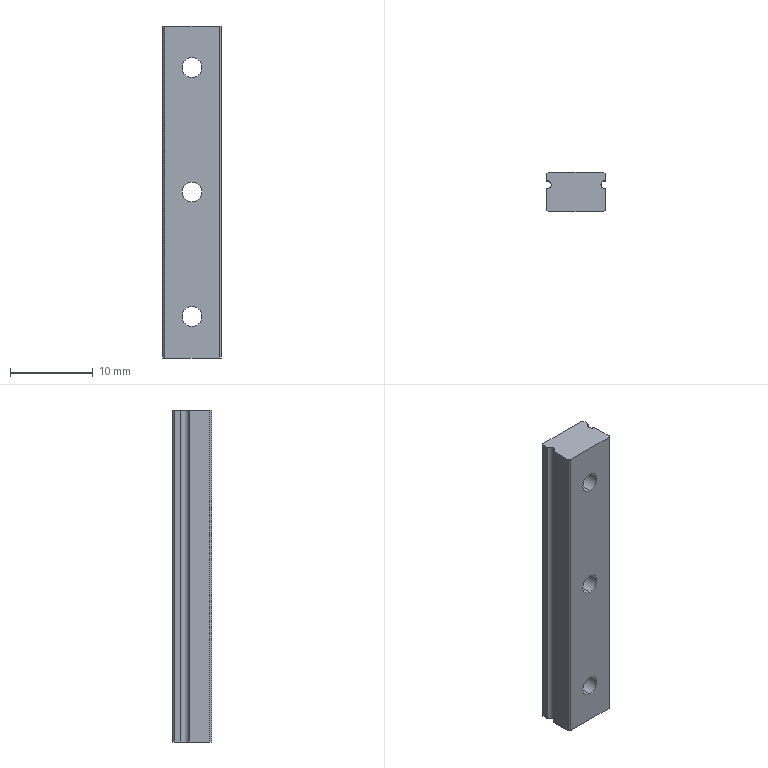Part | SolidWorks | features BaseBody 1 | 1 solid | 30 faces | box 7 x 4.7 x 40 mm | volume 1153 mm3 | cylinder 15 | plane 15 | commonest cylinder face diameters 2.4 x6 4.2 x6 1 x3
STEP:
#1=CARTESIAN_POINT('',(-8.978,1.895,33.8));
#2=VERTEX_POINT('',#1);
#3=CARTESIAN_POINT('',(-8.978,1.895,36.2));
#4=VERTEX_POINT('',#3);
#5=CARTESIAN_POINT('',(-8.978,1.895,35.));
#6=DIRECTION('',(0.,1.,0.));
#7=DIRECTION('',(0.,0.,1.));
#8=AXIS2_PLACEMENT_3D('',#5,#6,#7);
#9=CIRCLE('',#8,1.2);
#10=EDGE_CURVE('',#2,#4,#9,.T.);
#11=ORIENTED_EDGE('',*,*,#10,.F.);
#12=CARTESIAN_POINT('',(-8.978,4.295,33.8));
#13=VERTEX_POINT('',#12);
#14=CARTESIAN_POINT('',(-8.978,-34.284,33.8));
#15=DIRECTION('',(0.,1.,0.));
#16=VECTOR('',#15,1000.);
#17=LINE('',#14,#16);
#18=EDGE_CURVE('',#2,#13,#17,.T.);
#19=ORIENTED_EDGE('',*,*,#18,.T.);
#20=CARTESIAN_POINT('',(-8.978,4.295,36.2));
#21=VERTEX_POINT('',#20);
#22=CARTESIAN_POINT('',(-8.978,4.295,35.));
#23=DIRECTION('',(0.,-1.,0.));
#24=DIRECTION('',(0.,0.,1.));
#25=AXIS2_PLACEMENT_3D('',#22,#23,#24);
#26=CIRCLE('',#25,1.2);
#27=EDGE_CURVE('',#21,#13,#26,.T.);
#28=ORIENTED_EDGE('',*,*,#27,.F.);
#29=CARTESIAN_POINT('',(-8.978,-34.284,36.2));
#30=DIRECTION('',(0.,1.,0.));
#31=VECTOR('',#30,1000.);
#32=LINE('',#29,#31);
#33=EDGE_CURVE('',#4,#21,#32,.T.);
#34=ORIENTED_EDGE('',*,*,#33,.F.);
#35=EDGE_LOOP('',(#11,#19,#28,#34));
#36=FACE_OUTER_BOUND('',#35,.T.);
#37=CARTESIAN_POINT('',(-8.978,-34.284,35.));
#38=DIRECTION('',(0.,1.,0.));
#39=DIRECTION('',(0.,0.,1.));
#40=AXIS2_PLACEMENT_3D('',#37,#38,#39);
#41=CYLINDRICAL_SURFACE('',#40,1.2);
#42=ADVANCED_FACE('',(#36),#41,.F.);
#43=CARTESIAN_POINT('',(-8.978,1.895,18.8));
#44=VERTEX_POINT('',#43);
#45=CARTESIAN_POINT('',(-8.978,1.895,21.2));
#46=VERTEX_POINT('',#45);
#47=CARTESIAN_POINT('',(-8.978,1.895,20.));
#48=DIRECTION('',(0.,1.,0.));
#49=DIRECTION('',(0.,0.,1.));
#50=AXIS2_PLACEMENT_3D('',#47,#48,#49);
#51=CIRCLE('',#50,1.2);
#52=EDGE_CURVE('',#44,#46,#51,.T.);
#53=ORIENTED_EDGE('',*,*,#52,.F.);
#54=CARTESIAN_POINT('',(-8.978,4.295,18.8));
#55=VERTEX_POINT('',#54);
#56=CARTESIAN_POINT('',(-8.978,-34.284,18.8));
#57=DIRECTION('',(0.,1.,0.));
#58=VECTOR('',#57,1000.);
#59=LINE('',#56,#58);
#60=EDGE_CURVE('',#44,#55,#59,.T.);
#61=ORIENTED_EDGE('',*,*,#60,.T.);
#62=CARTESIAN_POINT('',(-8.978,4.295,21.2));
#63=VERTEX_POINT('',#62);
#64=CARTESIAN_POINT('',(-8.978,4.295,20.));
#65=DIRECTION('',(0.,-1.,0.));
#66=DIRECTION('',(0.,0.,1.));
#67=AXIS2_PLACEMENT_3D('',#64,#65,#66);
#68=CIRCLE('',#67,1.2);
#69=EDGE_CURVE('',#63,#55,#68,.T.);
#70=ORIENTED_EDGE('',*,*,#69,.F.);
#71=CARTESIAN_POINT('',(-8.978,-34.284,21.2));
#72=DIRECTION('',(0.,1.,0.));
#73=VECTOR('',#72,1000.);
#74=LINE('',#71,#73);
#75=EDGE_CURVE('',#46,#63,#74,.T.);
#76=ORIENTED_EDGE('',*,*,#75,.F.);
#77=EDGE_LOOP('',(#53,#61,#70,#76));
#78=FACE_OUTER_BOUND('',#77,.T.);
#79=CARTESIAN_POINT('',(-8.978,-34.284,20.));
#80=DIRECTION('',(0.,1.,0.));
#81=DIRECTION('',(0.,0.,1.));
#82=AXIS2_PLACEMENT_3D('',#79,#80,#81);
#83=CYLINDRICAL_SURFACE('',#82,1.2);
#84=ADVANCED_FACE('',(#78),#83,.F.);
#85=CARTESIAN_POINT('',(-8.978,1.895,3.8));
#86=VERTEX_POINT('',#85);
#87=CARTESIAN_POINT('',(-8.978,1.895,6.2));
#88=VERTEX_POINT('',#87);
#89=CARTESIAN_POINT('',(-8.978,1.895,5.));
#90=DIRECTION('',(0.,1.,0.));
#91=DIRECTION('',(0.,0.,1.));
#92=AXIS2_PLACEMENT_3D('',#89,#90,#91);
#93=CIRCLE('',#92,1.2);
#94=EDGE_CURVE('',#86,#88,#93,.T.);
#95=ORIENTED_EDGE('',*,*,#94,.F.);
#96=CARTESIAN_POINT('',(-8.978,4.295,3.8));
#97=VERTEX_POINT('',#96);
#98=CARTESIAN_POINT('',(-8.978,-34.284,3.8));
#99=DIRECTION('',(0.,1.,0.));
#100=VECTOR('',#99,1000.);
#101=LINE('',#98,#100);
#102=EDGE_CURVE('',#86,#97,#101,.T.);
#103=ORIENTED_EDGE('',*,*,#102,.T.);
#104=CARTESIAN_POINT('',(-8.978,4.295,6.2));
#105=VERTEX_POINT('',#104);
#106=CARTESIAN_POINT('',(-8.978,4.295,5.));
#107=DIRECTION('',(0.,-1.,0.));
#108=DIRECTION('',(0.,0.,1.));
#109=AXIS2_PLACEMENT_3D('',#106,#107,#108);
#110=CIRCLE('',#109,1.2);
#111=EDGE_CURVE('',#105,#97,#110,.T.);
#112=ORIENTED_EDGE('',*,*,#111,.F.);
#113=CARTESIAN_POINT('',(-8.978,-34.284,6.2));
#114=DIRECTION('',(0.,1.,0.));
#115=VECTOR('',#114,1000.);
#116=LINE('',#113,#115);
#117=EDGE_CURVE('',#88,#105,#116,.T.);
#118=ORIENTED_EDGE('',*,*,#117,.F.);
#119=EDGE_LOOP('',(#95,#103,#112,#118));
#120=FACE_OUTER_BOUND('',#119,.T.);
#121=CARTESIAN_POINT('',(-8.978,-34.284,5.));
#122=DIRECTION('',(0.,1.,0.));
#123=DIRECTION('',(0.,0.,1.));
#124=AXIS2_PLACEMENT_3D('',#121,#122,#123);
#125=CYLINDRICAL_SURFACE('',#124,1.2);
#126=ADVANCED_FACE('',(#120),#125,.F.);
#127=CARTESIAN_POINT('',(-8.978,4.295,32.9));
#128=VERTEX_POINT('',#127);
#129=CARTESIAN_POINT('',(-8.978,4.295,37.1));
#130=VERTEX_POINT('',#129);
#131=CARTESIAN_POINT('',(-8.978,4.295,35.));
#132=DIRECTION('',(0.,1.,0.));
#133=DIRECTION('',(0.,0.,1.));
#134=AXIS2_PLACEMENT_3D('',#131,#132,#133);
#135=CIRCLE('',#134,2.1);
#136=EDGE_CURVE('',#128,#130,#135,.T.);
#137=ORIENTED_EDGE('',*,*,#136,.F.);
#138=CARTESIAN_POINT('',(-8.978,6.595,32.9));
#139=VERTEX_POINT('',#138);
#140=CARTESIAN_POINT('',(-8.978,5.445,32.9));
#141=DIRECTION('',(0.,1.,0.));
#142=VECTOR('',#141,1000.);
#143=LINE('',#140,#142);
#144=EDGE_CURVE('',#128,#139,#143,.T.);
#145=ORIENTED_EDGE('',*,*,#144,.T.);
#146=CARTESIAN_POINT('',(-8.978,6.595,37.1));
#147=VERTEX_POINT('',#146);
#148=CARTESIAN_POINT('',(-8.978,6.595,35.));
#149=DIRECTION('',(0.,-1.,0.));
#150=DIRECTION('',(0.,0.,1.));
#151=AXIS2_PLACEMENT_3D('',#148,#149,#150);
#152=CIRCLE('',#151,2.1);
#153=EDGE_CURVE('',#147,#139,#152,.T.);
#154=ORIENTED_EDGE('',*,*,#153,.F.);
#155=CARTESIAN_POINT('',(-8.978,5.445,37.1));
#156=DIRECTION('',(0.,1.,0.));
#157=VECTOR('',#156,1000.);
#158=LINE('',#155,#157);
#159=EDGE_CURVE('',#130,#147,#158,.T.);
#160=ORIENTED_EDGE('',*,*,#159,.F.);
#161=EDGE_LOOP('',(#137,#145,#154,#160));
#162=FACE_OUTER_BOUND('',#161,.T.);
#163=CARTESIAN_POINT('',(-8.978,5.445,35.));
#164=DIRECTION('',(0.,1.,0.));
#165=DIRECTION('',(0.,0.,1.));
#166=AXIS2_PLACEMENT_3D('',#163,#164,#165);
#167=CYLINDRICAL_SURFACE('',#166,2.1);
#168=ADVANCED_FACE('',(#162),#167,.F.);
#169=CARTESIAN_POINT('',(-8.978,4.295,17.9));
#170=VERTEX_POINT('',#169);
#171=CARTESIAN_POINT('',(-8.978,4.295,22.1));
#172=VERTEX_POINT('',#171);
#173=CARTESIAN_POINT('',(-8.978,4.295,20.));
#174=DIRECTION('',(0.,1.,0.));
#175=DIRECTION('',(0.,0.,1.));
#176=AXIS2_PLACEMENT_3D('',#173,#174,#175);
#177=CIRCLE('',#176,2.1);
#178=EDGE_CURVE('',#170,#172,#177,.T.);
#179=ORIENTED_EDGE('',*,*,#178,.F.);
#180=CARTESIAN_POINT('',(-8.978,6.595,17.9));
#181=VERTEX_POINT('',#180);
#182=CARTESIAN_POINT('',(-8.978,5.445,17.9));
#183=DIRECTION('',(0.,1.,0.));
#184=VECTOR('',#183,1000.);
#185=LINE('',#182,#184);
#186=EDGE_CURVE('',#170,#181,#185,.T.);
#187=ORIENTED_EDGE('',*,*,#186,.T.);
#188=CARTESIAN_POINT('',(-8.978,6.595,22.1));
#189=VERTEX_POINT('',#188);
#190=CARTESIAN_POINT('',(-8.978,6.595,20.));
#191=DIRECTION('',(0.,-1.,0.));
#192=DIRECTION('',(0.,0.,1.));
#193=AXIS2_PLACEMENT_3D('',#190,#191,#192);
#194=CIRCLE('',#193,2.1);
#195=EDGE_CURVE('',#189,#181,#194,.T.);
#196=ORIENTED_EDGE('',*,*,#195,.F.);
#197=CARTESIAN_POINT('',(-8.978,5.445,22.1));
#198=DIRECTION('',(0.,1.,0.));
#199=VECTOR('',#198,1000.);
#200=LINE('',#197,#199);
#201=EDGE_CURVE('',#172,#189,#200,.T.);
#202=ORIENTED_EDGE('',*,*,#201,.F.);
#203=EDGE_LOOP('',(#179,#187,#196,#202));
#204=FACE_OUTER_BOUND('',#203,.T.);
#205=CARTESIAN_POINT('',(-8.978,5.445,20.));
#206=DIRECTION('',(0.,1.,0.));
#207=DIRECTION('',(0.,0.,1.));
#208=AXIS2_PLACEMENT_3D('',#205,#206,#207);
#209=CYLINDRICAL_SURFACE('',#208,2.1);
#210=ADVANCED_FACE('',(#204),#209,.F.);
#211=CARTESIAN_POINT('',(-8.978,4.295,2.9));
#212=VERTEX_POINT('',#211);
#213=CARTESIAN_POINT('',(-8.978,4.295,7.1));
#214=VERTEX_POINT('',#213);
#215=CARTESIAN_POINT('',(-8.978,4.295,5.));
#216=DIRECTION('',(0.,1.,0.));
#217=DIRECTION('',(0.,0.,1.));
#218=AXIS2_PLACEMENT_3D('',#215,#216,#217);
#219=CIRCLE('',#218,2.1);
#220=EDGE_CURVE('',#212,#214,#219,.T.);
#221=ORIENTED_EDGE('',*,*,#220,.F.);
#222=CARTESIAN_POINT('',(-8.978,6.595,2.9));
#223=VERTEX_POINT('',#222);
#224=CARTESIAN_POINT('',(-8.978,5.445,2.9));
#225=DIRECTION('',(0.,1.,0.));
#226=VECTOR('',#225,1000.);
#227=LINE('',#224,#226);
#228=EDGE_CURVE('',#212,#223,#227,.T.);
#229=ORIENTED_EDGE('',*,*,#228,.T.);
#230=CARTESIAN_POINT('',(-8.978,6.595,7.1));
#231=VERTEX_POINT('',#230);
#232=CARTESIAN_POINT('',(-8.978,6.595,5.));
#233=DIRECTION('',(0.,-1.,0.));
#234=DIRECTION('',(0.,0.,1.));
#235=AXIS2_PLACEMENT_3D('',#232,#233,#234);
#236=CIRCLE('',#235,2.1);
#237=EDGE_CURVE('',#231,#223,#236,.T.);
#238=ORIENTED_EDGE('',*,*,#237,.F.);
#239=CARTESIAN_POINT('',(-8.978,5.445,7.1));
#240=DIRECTION('',(0.,1.,0.));
#241=VECTOR('',#240,1000.);
#242=LINE('',#239,#241);
#243=EDGE_CURVE('',#214,#231,#242,.T.);
#244=ORIENTED_EDGE('',*,*,#243,.F.);
#245=EDGE_LOOP('',(#221,#229,#238,#244));
#246=FACE_OUTER_BOUND('',#245,.T.);
#247=CARTESIAN_POINT('',(-8.978,5.445,5.));
#248=DIRECTION('',(0.,1.,0.));
#249=DIRECTION('',(0.,0.,1.));
#250=AXIS2_PLACEMENT_3D('',#247,#248,#249);
#251=CYLINDRICAL_SURFACE('',#250,2.1);
#252=ADVANCED_FACE('',(#246),#251,.F.);
#253=CARTESIAN_POINT('',(-5.978,5.095,40.));
#254=VERTEX_POINT('',#253);
#255=CARTESIAN_POINT('',(-5.478,5.595,40.));
#256=VERTEX_POINT('',#255);
#257=CARTESIAN_POINT('',(-5.478,5.095,40.));
#258=DIRECTION('',(0.,0.,-1.));
#259=DIRECTION('',(-1.,0.,0.));
#260=AXIS2_PLACEMENT_3D('',#257,#258,#259);
#261=CIRCLE('',#260,0.5);
#262=EDGE_CURVE('',#254,#256,#261,.T.);
#263=ORIENTED_EDGE('',*,*,#262,.F.);
#264=CARTESIAN_POINT('',(-5.978,5.095,0.));
#265=VERTEX_POINT('',#264);
#266=CARTESIAN_POINT('',(-5.978,5.095,40.));
#267=DIRECTION('',(0.,0.,-1.));
#268=VECTOR('',#267,1000.);
#269=LINE('',#266,#268);
#270=EDGE_CURVE('',#254,#265,#269,.T.);
#271=ORIENTED_EDGE('',*,*,#270,.T.);
#272=CARTESIAN_POINT('',(-5.478,5.595,0.));
#273=VERTEX_POINT('',#272);
#274=CARTESIAN_POINT('',(-5.478,5.095,0.));
#275=DIRECTION('',(0.,0.,1.));
#276=DIRECTION('',(-1.,0.,0.));
#277=AXIS2_PLACEMENT_3D('',#274,#275,#276);
#278=CIRCLE('',#277,0.5);
#279=EDGE_CURVE('',#273,#265,#278,.T.);
#280=ORIENTED_EDGE('',*,*,#279,.F.);
#281=CARTESIAN_POINT('',(-5.478,5.595,40.));
#282=DIRECTION('',(0.,0.,-1.));
#283=VECTOR('',#282,1000.);
#284=LINE('',#281,#283);
#285=EDGE_CURVE('',#256,#273,#284,.T.);
#286=ORIENTED_EDGE('',*,*,#285,.F.);
#287=EDGE_LOOP('',(#263,#271,#280,#286));
#288=FACE_OUTER_BOUND('',#287,.T.);
#289=CARTESIAN_POINT('',(-5.478,5.095,40.));
#290=DIRECTION('',(0.,0.,-1.));
#291=DIRECTION('',(-1.,0.,0.));
#292=AXIS2_PLACEMENT_3D('',#289,#290,#291);
#293=CYLINDRICAL_SURFACE('',#292,0.5);
#294=ADVANCED_FACE('',(#288),#293,.F.);
#295=CARTESIAN_POINT('',(-8.978,1.895,35.));
#296=DIRECTION('',(0.,1.,0.));
#297=DIRECTION('',(0.,0.,1.));
#298=AXIS2_PLACEMENT_3D('',#295,#296,#297);
#299=CIRCLE('',#298,1.2);
#300=EDGE_CURVE('',#4,#2,#299,.T.);
#301=ORIENTED_EDGE('',*,*,#300,.T.);
#302=ORIENTED_EDGE('',*,*,#10,.T.);
#303=EDGE_LOOP('',(#301,#302));
#304=FACE_BOUND('',#303,.T.);
#305=CARTESIAN_POINT('',(-8.978,1.895,20.));
#306=DIRECTION('',(0.,1.,0.));
#307=DIRECTION('',(0.,0.,1.));
#308=AXIS2_PLACEMENT_3D('',#305,#306,#307);
#309=CIRCLE('',#308,1.2);
#310=EDGE_CURVE('',#46,#44,#309,.T.);
#311=ORIENTED_EDGE('',*,*,#310,.T.);
#312=ORIENTED_EDGE('',*,*,#52,.T.);
#313=EDGE_LOOP('',(#311,#312));
#314=FACE_BOUND('',#313,.T.);
#315=CARTESIAN_POINT('',(-8.978,1.895,5.));
#316=DIRECTION('',(0.,1.,0.));
#317=DIRECTION('',(0.,0.,1.));
#318=AXIS2_PLACEMENT_3D('',#315,#316,#317);
#319=CIRCLE('',#318,1.2);
#320=EDGE_CURVE('',#88,#86,#319,.T.);
#321=ORIENTED_EDGE('',*,*,#320,.T.);
#322=ORIENTED_EDGE('',*,*,#94,.T.);
#323=EDGE_LOOP('',(#321,#322));
#324=FACE_BOUND('',#323,.T.);
#325=CARTESIAN_POINT('',(-12.278,1.895,40.));
#326=VERTEX_POINT('',#325);
#327=CARTESIAN_POINT('',(-12.278,1.895,0.));
#328=VERTEX_POINT('',#327);
#329=CARTESIAN_POINT('',(-12.278,1.895,0.));
#330=DIRECTION('',(0.,0.,-1.));
#331=VECTOR('',#330,1000.);
#332=LINE('',#329,#331);
#333=EDGE_CURVE('',#326,#328,#332,.T.);
#334=ORIENTED_EDGE('',*,*,#333,.T.);
#335=CARTESIAN_POINT('',(-5.678,1.895,0.));
#336=VERTEX_POINT('',#335);
#337=CARTESIAN_POINT('',(-5.478,1.895,0.));
#338=DIRECTION('',(1.,0.,0.));
#339=VECTOR('',#338,1000.);
#340=LINE('',#337,#339);
#341=EDGE_CURVE('',#328,#336,#340,.T.);
#342=ORIENTED_EDGE('',*,*,#341,.T.);
#343=CARTESIAN_POINT('',(-5.678,1.895,40.));
#344=VERTEX_POINT('',#343);
#345=CARTESIAN_POINT('',(-5.678,1.895,0.));
#346=DIRECTION('',(0.,0.,1.));
#347=VECTOR('',#346,1000.);
#348=LINE('',#345,#347);
#349=EDGE_CURVE('',#336,#344,#348,.T.);
#350=ORIENTED_EDGE('',*,*,#349,.T.);
#351=CARTESIAN_POINT('',(-5.478,1.895,40.));
#352=DIRECTION('',(-1.,0.,0.));
#353=VECTOR('',#352,1000.);
#354=LINE('',#351,#353);
#355=EDGE_CURVE('',#344,#326,#354,.T.);
#356=ORIENTED_EDGE('',*,*,#355,.T.);
#357=EDGE_LOOP('',(#334,#342,#350,#356));
#358=FACE_OUTER_BOUND('',#357,.T.);
#359=CARTESIAN_POINT('',(-5.478,1.895,0.));
#360=DIRECTION('',(0.,-1.,0.));
#361=DIRECTION('',(0.,0.,-1.));
#362=AXIS2_PLACEMENT_3D('',#359,#360,#361);
#363=PLANE('',#362);
#364=ADVANCED_FACE('',(#304,#314,#324,#358),#363,.T.);
#365=ORIENTED_EDGE('',*,*,#18,.F.);
#366=ORIENTED_EDGE('',*,*,#300,.F.);
#367=ORIENTED_EDGE('',*,*,#33,.T.);
#368=CARTESIAN_POINT('',(-8.978,4.295,35.));
#369=DIRECTION('',(0.,-1.,0.));
#370=DIRECTION('',(0.,0.,1.));
#371=AXIS2_PLACEMENT_3D('',#368,#369,#370);
#372=CIRCLE('',#371,1.2);
#373=EDGE_CURVE('',#13,#21,#372,.T.);
#374=ORIENTED_EDGE('',*,*,#373,.F.);
#375=EDGE_LOOP('',(#365,#366,#367,#374));
#376=FACE_OUTER_BOUND('',#375,.T.);
#377=CARTESIAN_POINT('',(-8.978,-34.284,35.));
#378=DIRECTION('',(0.,1.,0.));
#379=DIRECTION('',(0.,0.,1.));
#380=AXIS2_PLACEMENT_3D('',#377,#378,#379);
#381=CYLINDRICAL_SURFACE('',#380,1.2);
#382=ADVANCED_FACE('',(#376),#381,.F.);
#383=ORIENTED_EDGE('',*,*,#60,.F.);
#384=ORIENTED_EDGE('',*,*,#310,.F.);
#385=ORIENTED_EDGE('',*,*,#75,.T.);
#386=CARTESIAN_POINT('',(-8.978,4.295,20.));
#387=DIRECTION('',(0.,-1.,0.));
#388=DIRECTION('',(0.,0.,1.));
#389=AXIS2_PLACEMENT_3D('',#386,#387,#388);
#390=CIRCLE('',#389,1.2);
#391=EDGE_CURVE('',#55,#63,#390,.T.);
#392=ORIENTED_EDGE('',*,*,#391,.F.);
#393=EDGE_LOOP('',(#383,#384,#385,#392));
#394=FACE_OUTER_BOUND('',#393,.T.);
#395=CARTESIAN_POINT('',(-8.978,-34.284,20.));
#396=DIRECTION('',(0.,1.,0.));
#397=DIRECTION('',(0.,0.,1.));
#398=AXIS2_PLACEMENT_3D('',#395,#396,#397);
#399=CYLINDRICAL_SURFACE('',#398,1.2);
#400=ADVANCED_FACE('',(#394),#399,.F.);
#401=ORIENTED_EDGE('',*,*,#102,.F.);
#402=ORIENTED_EDGE('',*,*,#320,.F.);
#403=ORIENTED_EDGE('',*,*,#117,.T.);
#404=CARTESIAN_POINT('',(-8.978,4.295,5.));
#405=DIRECTION('',(0.,-1.,0.));
#406=DIRECTION('',(0.,0.,1.));
#407=AXIS2_PLACEMENT_3D('',#404,#405,#406);
#408=CIRCLE('',#407,1.2);
#409=EDGE_CURVE('',#97,#105,#408,.T.);
#410=ORIENTED_EDGE('',*,*,#409,.F.);
#411=EDGE_LOOP('',(#401,#402,#403,#410));
#412=FACE_OUTER_BOUND('',#411,.T.);
#413=CARTESIAN_POINT('',(-8.978,-34.284,5.));
#414=DIRECTION('',(0.,1.,0.));
#415=DIRECTION('',(0.,0.,1.));
#416=AXIS2_PLACEMENT_3D('',#413,#414,#415);
#417=CYLINDRICAL_SURFACE('',#416,1.2);
#418=ADVANCED_FACE('',(#412),#417,.F.);
#419=ORIENTED_EDGE('',*,*,#341,.F.);
#420=CARTESIAN_POINT('',(-12.478,2.095,0.));
#421=VERTEX_POINT('',#420);
#422=CARTESIAN_POINT('',(-12.478,2.095,0.));
#423=DIRECTION('',(0.7071,-0.7071,0.));
#424=VECTOR('',#423,1000.);
#425=LINE('',#422,#424);
#426=EDGE_CURVE('',#421,#328,#425,.T.);
#427=ORIENTED_EDGE('',*,*,#426,.F.);
#428=CARTESIAN_POINT('',(-12.478,4.595,0.));
#429=VERTEX_POINT('',#428);
#430=CARTESIAN_POINT('',(-12.478,4.245,0.));
#431=DIRECTION('',(0.,-1.,0.));
#432=VECTOR('',#431,1000.);
#433=LINE('',#430,#432);
#434=EDGE_CURVE('',#429,#421,#433,.T.);
#435=ORIENTED_EDGE('',*,*,#434,.F.);
#436=CARTESIAN_POINT('',(-12.478,5.595,0.));
#437=VERTEX_POINT('',#436);
#438=CARTESIAN_POINT('',(-12.478,5.095,0.));
#439=DIRECTION('',(0.,0.,1.));
#440=DIRECTION('',(-1.,0.,0.));
#441=AXIS2_PLACEMENT_3D('',#438,#439,#440);
#442=CIRCLE('',#441,0.5);
#443=EDGE_CURVE('',#429,#437,#442,.T.);
#444=ORIENTED_EDGE('',*,*,#443,.T.);
#445=CARTESIAN_POINT('',(-12.478,6.395,0.));
#446=VERTEX_POINT('',#445);
#447=CARTESIAN_POINT('',(-12.478,1.895,0.));
#448=DIRECTION('',(0.,-1.,0.));
#449=VECTOR('',#448,1000.);
#450=LINE('',#447,#449);
#451=EDGE_CURVE('',#446,#437,#450,.T.);
#452=ORIENTED_EDGE('',*,*,#451,.F.);
#453=CARTESIAN_POINT('',(-12.278,6.595,0.));
#454=VERTEX_POINT('',#453);
#455=CARTESIAN_POINT('',(-12.378,6.495,0.));
#456=DIRECTION('',(-0.7071,-0.7071,0.));
#457=VECTOR('',#456,1000.);
#458=LINE('',#455,#457);
#459=EDGE_CURVE('',#454,#446,#458,.T.);
#460=ORIENTED_EDGE('',*,*,#459,.F.);
#461=CARTESIAN_POINT('',(-5.678,6.595,0.));
#462=VERTEX_POINT('',#461);
#463=CARTESIAN_POINT('',(-8.978,6.595,0.));
#464=DIRECTION('',(-1.,0.,0.));
#465=VECTOR('',#464,1000.);
#466=LINE('',#463,#465);
#467=EDGE_CURVE('',#462,#454,#466,.T.);
#468=ORIENTED_EDGE('',*,*,#467,.F.);
#469=CARTESIAN_POINT('',(-5.478,6.395,0.));
#470=VERTEX_POINT('',#469);
#471=CARTESIAN_POINT('',(-5.578,6.495,0.));
#472=DIRECTION('',(-0.7071,0.7071,0.));
#473=VECTOR('',#472,1000.);
#474=LINE('',#471,#473);
#475=EDGE_CURVE('',#470,#462,#474,.T.);
#476=ORIENTED_EDGE('',*,*,#475,.F.);
#477=CARTESIAN_POINT('',(-5.478,6.595,0.));
#478=DIRECTION('',(0.,1.,0.));
#479=VECTOR('',#478,1000.);
#480=LINE('',#477,#479);
#481=EDGE_CURVE('',#273,#470,#480,.T.);
#482=ORIENTED_EDGE('',*,*,#481,.F.);
#483=ORIENTED_EDGE('',*,*,#279,.T.);
#484=CARTESIAN_POINT('',(-5.478,4.595,0.));
#485=VERTEX_POINT('',#484);
#486=CARTESIAN_POINT('',(-5.478,5.095,0.));
#487=DIRECTION('',(0.,0.,1.));
#488=DIRECTION('',(-1.,0.,0.));
#489=AXIS2_PLACEMENT_3D('',#486,#487,#488);
#490=CIRCLE('',#489,0.5);
#491=EDGE_CURVE('',#265,#485,#490,.T.);
#492=ORIENTED_EDGE('',*,*,#491,.T.);
#493=CARTESIAN_POINT('',(-5.478,2.095,0.));
#494=VERTEX_POINT('',#493);
#495=CARTESIAN_POINT('',(-5.478,4.245,0.));
#496=DIRECTION('',(0.,1.,0.));
#497=VECTOR('',#496,1000.);
#498=LINE('',#495,#497);
#499=EDGE_CURVE('',#494,#485,#498,.T.);
#500=ORIENTED_EDGE('',*,*,#499,.F.);
#501=CARTESIAN_POINT('',(-5.678,1.895,0.));
#502=DIRECTION('',(0.7071,0.7071,0.));
#503=VECTOR('',#502,1000.);
#504=LINE('',#501,#503);
#505=EDGE_CURVE('',#336,#494,#504,.T.);
#506=ORIENTED_EDGE('',*,*,#505,.F.);
#507=EDGE_LOOP('',(#419,#427,#435,#444,#452,#460,#468,#476,#482,#483,#492,#500,#506));
#508=FACE_OUTER_BOUND('',#507,.T.);
#509=CARTESIAN_POINT('',(-8.978,4.245,0.));
#510=DIRECTION('',(0.,0.,1.));
#511=DIRECTION('',(1.,0.,0.));
#512=AXIS2_PLACEMENT_3D('',#509,#510,#511);
#513=PLANE('',#512);
#514=ADVANCED_FACE('',(#508),#513,.F.);
#515=ORIENTED_EDGE('',*,*,#426,.T.);
#516=ORIENTED_EDGE('',*,*,#333,.F.);
#517=CARTESIAN_POINT('',(-12.478,2.095,40.));
#518=VERTEX_POINT('',#517);
#519=CARTESIAN_POINT('',(-12.378,1.995,40.));
#520=DIRECTION('',(-0.7071,0.7071,0.));
#521=VECTOR('',#520,1000.);
#522=LINE('',#519,#521);
#523=EDGE_CURVE('',#326,#518,#522,.T.);
#524=ORIENTED_EDGE('',*,*,#523,.T.);
#525=CARTESIAN_POINT('',(-12.478,2.095,0.));
#526=DIRECTION('',(0.,0.,-1.));
#527=VECTOR('',#526,1000.);
#528=LINE('',#525,#527);
#529=EDGE_CURVE('',#518,#421,#528,.T.);
#530=ORIENTED_EDGE('',*,*,#529,.T.);
#531=EDGE_LOOP('',(#515,#516,#524,#530));
#532=FACE_OUTER_BOUND('',#531,.T.);
#533=CARTESIAN_POINT('',(-12.378,1.995,0.));
#534=DIRECTION('',(-0.7071,-0.7071,0.));
#535=DIRECTION('',(0.7071,-0.7071,0.));
#536=AXIS2_PLACEMENT_3D('',#533,#534,#535);
#537=PLANE('',#536);
#538=ADVANCED_FACE('',(#532),#537,.T.);
#539=ORIENTED_EDGE('',*,*,#523,.F.);
#540=ORIENTED_EDGE('',*,*,#355,.F.);
#541=CARTESIAN_POINT('',(-5.478,2.095,40.));
#542=VERTEX_POINT('',#541);
#543=CARTESIAN_POINT('',(-5.678,1.895,40.));
#544=DIRECTION('',(0.7071,0.7071,0.));
#545=VECTOR('',#544,1000.);
#546=LINE('',#543,#545);
#547=EDGE_CURVE('',#344,#542,#546,.T.);
#548=ORIENTED_EDGE('',*,*,#547,.T.);
#549=CARTESIAN_POINT('',(-5.478,4.595,40.));
#550=VERTEX_POINT('',#549);
#551=CARTESIAN_POINT('',(-5.478,4.245,40.));
#552=DIRECTION('',(0.,1.,0.));
#553=VECTOR('',#552,1000.);
#554=LINE('',#551,#553);
#555=EDGE_CURVE('',#542,#550,#554,.T.);
#556=ORIENTED_EDGE('',*,*,#555,.T.);
#557=CARTESIAN_POINT('',(-5.478,5.095,40.));
#558=DIRECTION('',(0.,0.,-1.));
#559=DIRECTION('',(-1.,0.,0.));
#560=AXIS2_PLACEMENT_3D('',#557,#558,#559);
#561=CIRCLE('',#560,0.5);
#562=EDGE_CURVE('',#550,#254,#561,.T.);
#563=ORIENTED_EDGE('',*,*,#562,.T.);
#564=ORIENTED_EDGE('',*,*,#262,.T.);
#565=CARTESIAN_POINT('',(-5.478,6.395,40.));
#566=VERTEX_POINT('',#565);
#567=CARTESIAN_POINT('',(-5.478,6.595,40.));
#568=DIRECTION('',(0.,-1.,0.));
#569=VECTOR('',#568,1000.);
#570=LINE('',#567,#569);
#571=EDGE_CURVE('',#566,#256,#570,.T.);
#572=ORIENTED_EDGE('',*,*,#571,.F.);
#573=CARTESIAN_POINT('',(-5.678,6.595,40.));
#574=VERTEX_POINT('',#573);
#575=CARTESIAN_POINT('',(-5.578,6.495,40.));
#576=DIRECTION('',(0.7071,-0.7071,0.));
#577=VECTOR('',#576,1000.);
#578=LINE('',#575,#577);
#579=EDGE_CURVE('',#574,#566,#578,.T.);
#580=ORIENTED_EDGE('',*,*,#579,.F.);
#581=CARTESIAN_POINT('',(-12.278,6.595,40.));
#582=VERTEX_POINT('',#581);
#583=CARTESIAN_POINT('',(-8.978,6.595,40.));
#584=DIRECTION('',(-1.,0.,0.));
#585=VECTOR('',#584,1000.);
#586=LINE('',#583,#585);
#587=EDGE_CURVE('',#574,#582,#586,.T.);
#588=ORIENTED_EDGE('',*,*,#587,.T.);
#589=CARTESIAN_POINT('',(-12.478,6.395,40.));
#590=VERTEX_POINT('',#589);
#591=CARTESIAN_POINT('',(-12.378,6.495,40.));
#592=DIRECTION('',(0.7071,0.7071,0.));
#593=VECTOR('',#592,1000.);
#594=LINE('',#591,#593);
#595=EDGE_CURVE('',#590,#582,#594,.T.);
#596=ORIENTED_EDGE('',*,*,#595,.F.);
#597=CARTESIAN_POINT('',(-12.478,5.595,40.));
#598=VERTEX_POINT('',#597);
#599=CARTESIAN_POINT('',(-12.478,1.895,40.));
#600=DIRECTION('',(0.,1.,0.));
#601=VECTOR('',#600,1000.);
#602=LINE('',#599,#601);
#603=EDGE_CURVE('',#598,#590,#602,.T.);
#604=ORIENTED_EDGE('',*,*,#603,.F.);
#605=CARTESIAN_POINT('',(-12.478,4.595,40.));
#606=VERTEX_POINT('',#605);
#607=CARTESIAN_POINT('',(-12.478,5.095,40.));
#608=DIRECTION('',(0.,0.,-1.));
#609=DIRECTION('',(-1.,0.,0.));
#610=AXIS2_PLACEMENT_3D('',#607,#608,#609);
#611=CIRCLE('',#610,0.5);
#612=EDGE_CURVE('',#598,#606,#611,.T.);
#613=ORIENTED_EDGE('',*,*,#612,.T.);
#614=CARTESIAN_POINT('',(-12.478,4.245,40.));
#615=DIRECTION('',(0.,-1.,0.));
#616=VECTOR('',#615,1000.);
#617=LINE('',#614,#616);
#618=EDGE_CURVE('',#606,#518,#617,.T.);
#619=ORIENTED_EDGE('',*,*,#618,.T.);
#620=EDGE_LOOP('',(#539,#540,#548,#556,#563,#564,#572,#580,#588,#596,#604,#613,#619));
#621=FACE_OUTER_BOUND('',#620,.T.);
#622=CARTESIAN_POINT('',(-8.978,4.245,40.));
#623=DIRECTION('',(0.,0.,1.));
#624=DIRECTION('',(1.,0.,0.));
#625=AXIS2_PLACEMENT_3D('',#622,#623,#624);
#626=PLANE('',#625);
#627=ADVANCED_FACE('',(#621),#626,.T.);
#628=ORIENTED_EDGE('',*,*,#505,.T.);
#629=CARTESIAN_POINT('',(-5.478,2.095,0.));
#630=DIRECTION('',(0.,0.,1.));
#631=VECTOR('',#630,1000.);
#632=LINE('',#629,#631);
#633=EDGE_CURVE('',#494,#542,#632,.T.);
#634=ORIENTED_EDGE('',*,*,#633,.T.);
#635=ORIENTED_EDGE('',*,*,#547,.F.);
#636=ORIENTED_EDGE('',*,*,#349,.F.);
#637=EDGE_LOOP('',(#628,#634,#635,#636));
#638=FACE_OUTER_BOUND('',#637,.T.);
#639=CARTESIAN_POINT('',(-5.578,1.995,0.));
#640=DIRECTION('',(0.7071,-0.7071,0.));
#641=DIRECTION('',(0.7071,0.7071,0.));
#642=AXIS2_PLACEMENT_3D('',#639,#640,#641);
#643=PLANE('',#642);
#644=ADVANCED_FACE('',(#638),#643,.T.);
#645=ORIENTED_EDGE('',*,*,#27,.T.);
#646=ORIENTED_EDGE('',*,*,#373,.T.);
#647=EDGE_LOOP('',(#645,#646));
#648=FACE_BOUND('',#647,.T.);
#649=CARTESIAN_POINT('',(-8.978,4.295,35.));
#650=DIRECTION('',(0.,1.,0.));
#651=DIRECTION('',(0.,0.,1.));
#652=AXIS2_PLACEMENT_3D('',#649,#650,#651);
#653=CIRCLE('',#652,2.1);
#654=EDGE_CURVE('',#130,#128,#653,.T.);
#655=ORIENTED_EDGE('',*,*,#654,.T.);
#656=ORIENTED_EDGE('',*,*,#136,.T.);
#657=EDGE_LOOP('',(#655,#656));
#658=FACE_OUTER_BOUND('',#657,.T.);
#659=CARTESIAN_POINT('',(-8.978,4.295,35.));
#660=DIRECTION('',(0.,1.,0.));
#661=DIRECTION('',(0.,0.,1.));
#662=AXIS2_PLACEMENT_3D('',#659,#660,#661);
#663=PLANE('',#662);
#664=ADVANCED_FACE('',(#648,#658),#663,.T.);
#665=ORIENTED_EDGE('',*,*,#69,.T.);
#666=ORIENTED_EDGE('',*,*,#391,.T.);
#667=EDGE_LOOP('',(#665,#666));
#668=FACE_BOUND('',#667,.T.);
#669=CARTESIAN_POINT('',(-8.978,4.295,20.));
#670=DIRECTION('',(0.,1.,0.));
#671=DIRECTION('',(0.,0.,1.));
#672=AXIS2_PLACEMENT_3D('',#669,#670,#671);
#673=CIRCLE('',#672,2.1);
#674=EDGE_CURVE('',#172,#170,#673,.T.);
#675=ORIENTED_EDGE('',*,*,#674,.T.);
#676=ORIENTED_EDGE('',*,*,#178,.T.);
#677=EDGE_LOOP('',(#675,#676));
#678=FACE_OUTER_BOUND('',#677,.T.);
#679=CARTESIAN_POINT('',(-8.978,4.295,20.));
#680=DIRECTION('',(0.,1.,0.));
#681=DIRECTION('',(0.,0.,1.));
#682=AXIS2_PLACEMENT_3D('',#679,#680,#681);
#683=PLANE('',#682);
#684=ADVANCED_FACE('',(#668,#678),#683,.T.);
#685=ORIENTED_EDGE('',*,*,#111,.T.);
#686=ORIENTED_EDGE('',*,*,#409,.T.);
#687=EDGE_LOOP('',(#685,#686));
#688=FACE_BOUND('',#687,.T.);
#689=CARTESIAN_POINT('',(-8.978,4.295,5.));
#690=DIRECTION('',(0.,1.,0.));
#691=DIRECTION('',(0.,0.,1.));
#692=AXIS2_PLACEMENT_3D('',#689,#690,#691);
#693=CIRCLE('',#692,2.1);
#694=EDGE_CURVE('',#214,#212,#693,.T.);
#695=ORIENTED_EDGE('',*,*,#694,.T.);
#696=ORIENTED_EDGE('',*,*,#220,.T.);
#697=EDGE_LOOP('',(#695,#696));
#698=FACE_OUTER_BOUND('',#697,.T.);
#699=CARTESIAN_POINT('',(-8.978,4.295,5.));
#700=DIRECTION('',(0.,1.,0.));
#701=DIRECTION('',(0.,0.,1.));
#702=AXIS2_PLACEMENT_3D('',#699,#700,#701);
#703=PLANE('',#702);
#704=ADVANCED_FACE('',(#688,#698),#703,.T.);
#705=CARTESIAN_POINT('',(-12.478,4.595,0.));
#706=DIRECTION('',(0.,0.,-1.));
#707=VECTOR('',#706,1000.);
#708=LINE('',#705,#707);
#709=EDGE_CURVE('',#606,#429,#708,.T.);
#710=ORIENTED_EDGE('',*,*,#709,.T.);
#711=ORIENTED_EDGE('',*,*,#434,.T.);
#712=ORIENTED_EDGE('',*,*,#529,.F.);
#713=ORIENTED_EDGE('',*,*,#618,.F.);
#714=EDGE_LOOP('',(#710,#711,#712,#713));
#715=FACE_OUTER_BOUND('',#714,.T.);
#716=CARTESIAN_POINT('',(-12.478,1.895,0.));
#717=DIRECTION('',(-1.,0.,0.));
#718=DIRECTION('',(0.,0.,1.));
#719=AXIS2_PLACEMENT_3D('',#716,#717,#718);
#720=PLANE('',#719);
#721=ADVANCED_FACE('',(#715),#720,.T.);
#722=ORIENTED_EDGE('',*,*,#153,.T.);
#723=CARTESIAN_POINT('',(-8.978,6.595,35.));
#724=DIRECTION('',(0.,-1.,0.));
#725=DIRECTION('',(0.,0.,1.));
#726=AXIS2_PLACEMENT_3D('',#723,#724,#725);
#727=CIRCLE('',#726,2.1);
#728=EDGE_CURVE('',#139,#147,#727,.T.);
#729=ORIENTED_EDGE('',*,*,#728,.T.);
#730=EDGE_LOOP('',(#722,#729));
#731=FACE_BOUND('',#730,.T.);
#732=ORIENTED_EDGE('',*,*,#195,.T.);
#733=CARTESIAN_POINT('',(-8.978,6.595,20.));
#734=DIRECTION('',(0.,-1.,0.));
#735=DIRECTION('',(0.,0.,1.));
#736=AXIS2_PLACEMENT_3D('',#733,#734,#735);
#737=CIRCLE('',#736,2.1);
#738=EDGE_CURVE('',#181,#189,#737,.T.);
#739=ORIENTED_EDGE('',*,*,#738,.T.);
#740=EDGE_LOOP('',(#732,#739));
#741=FACE_BOUND('',#740,.T.);
#742=ORIENTED_EDGE('',*,*,#237,.T.);
#743=CARTESIAN_POINT('',(-8.978,6.595,5.));
#744=DIRECTION('',(0.,-1.,0.));
#745=DIRECTION('',(0.,0.,1.));
#746=AXIS2_PLACEMENT_3D('',#743,#744,#745);
#747=CIRCLE('',#746,2.1);
#748=EDGE_CURVE('',#223,#231,#747,.T.);
#749=ORIENTED_EDGE('',*,*,#748,.T.);
#750=EDGE_LOOP('',(#742,#749));
#751=FACE_BOUND('',#750,.T.);
#752=CARTESIAN_POINT('',(-12.278,6.595,0.));
#753=DIRECTION('',(0.,0.,1.));
#754=VECTOR('',#753,1000.);
#755=LINE('',#752,#754);
#756=EDGE_CURVE('',#454,#582,#755,.T.);
#757=ORIENTED_EDGE('',*,*,#756,.T.);
#758=ORIENTED_EDGE('',*,*,#587,.F.);
#759=CARTESIAN_POINT('',(-5.678,6.595,0.));
#760=DIRECTION('',(0.,0.,-1.));
#761=VECTOR('',#760,1000.);
#762=LINE('',#759,#761);
#763=EDGE_CURVE('',#574,#462,#762,.T.);
#764=ORIENTED_EDGE('',*,*,#763,.T.);
#765=ORIENTED_EDGE('',*,*,#467,.T.);
#766=EDGE_LOOP('',(#757,#758,#764,#765));
#767=FACE_OUTER_BOUND('',#766,.T.);
#768=CARTESIAN_POINT('',(-12.478,6.595,0.));
#769=DIRECTION('',(0.,1.,0.));
#770=DIRECTION('',(0.,0.,1.));
#771=AXIS2_PLACEMENT_3D('',#768,#769,#770);
#772=PLANE('',#771);
#773=ADVANCED_FACE('',(#731,#741,#751,#767),#772,.T.);
#774=CARTESIAN_POINT('',(-5.478,4.595,0.));
#775=DIRECTION('',(0.,0.,1.));
#776=VECTOR('',#775,1000.);
#777=LINE('',#774,#776);
#778=EDGE_CURVE('',#485,#550,#777,.T.);
#779=ORIENTED_EDGE('',*,*,#778,.T.);
#780=ORIENTED_EDGE('',*,*,#555,.F.);
#781=ORIENTED_EDGE('',*,*,#633,.F.);
#782=ORIENTED_EDGE('',*,*,#499,.T.);
#783=EDGE_LOOP('',(#779,#780,#781,#782));
#784=FACE_OUTER_BOUND('',#783,.T.);
#785=CARTESIAN_POINT('',(-5.478,6.595,0.));
#786=DIRECTION('',(1.,0.,0.));
#787=DIRECTION('',(0.,0.,-1.));
#788=AXIS2_PLACEMENT_3D('',#785,#786,#787);
#789=PLANE('',#788);
#790=ADVANCED_FACE('',(#784),#789,.T.);
#791=ORIENTED_EDGE('',*,*,#144,.F.);
#792=ORIENTED_EDGE('',*,*,#654,.F.);
#793=ORIENTED_EDGE('',*,*,#159,.T.);
#794=ORIENTED_EDGE('',*,*,#728,.F.);
#795=EDGE_LOOP('',(#791,#792,#793,#794));
#796=FACE_OUTER_BOUND('',#795,.T.);
#797=CARTESIAN_POINT('',(-8.978,5.445,35.));
#798=DIRECTION('',(0.,1.,0.));
#799=DIRECTION('',(0.,0.,1.));
#800=AXIS2_PLACEMENT_3D('',#797,#798,#799);
#801=CYLINDRICAL_SURFACE('',#800,2.1);
#802=ADVANCED_FACE('',(#796),#801,.F.);
#803=ORIENTED_EDGE('',*,*,#186,.F.);
#804=ORIENTED_EDGE('',*,*,#674,.F.);
#805=ORIENTED_EDGE('',*,*,#201,.T.);
#806=ORIENTED_EDGE('',*,*,#738,.F.);
#807=EDGE_LOOP('',(#803,#804,#805,#806));
#808=FACE_OUTER_BOUND('',#807,.T.);
#809=CARTESIAN_POINT('',(-8.978,5.445,20.));
#810=DIRECTION('',(0.,1.,0.));
#811=DIRECTION('',(0.,0.,1.));
#812=AXIS2_PLACEMENT_3D('',#809,#810,#811);
#813=CYLINDRICAL_SURFACE('',#812,2.1);
#814=ADVANCED_FACE('',(#808),#813,.F.);
#815=ORIENTED_EDGE('',*,*,#228,.F.);
#816=ORIENTED_EDGE('',*,*,#694,.F.);
#817=ORIENTED_EDGE('',*,*,#243,.T.);
#818=ORIENTED_EDGE('',*,*,#748,.F.);
#819=EDGE_LOOP('',(#815,#816,#817,#818));
#820=FACE_OUTER_BOUND('',#819,.T.);
#821=CARTESIAN_POINT('',(-8.978,5.445,5.));
#822=DIRECTION('',(0.,1.,0.));
#823=DIRECTION('',(0.,0.,1.));
#824=AXIS2_PLACEMENT_3D('',#821,#822,#823);
#825=CYLINDRICAL_SURFACE('',#824,2.1);
#826=ADVANCED_FACE('',(#820),#825,.F.);
#827=ORIENTED_EDGE('',*,*,#443,.F.);
#828=ORIENTED_EDGE('',*,*,#709,.F.);
#829=ORIENTED_EDGE('',*,*,#612,.F.);
#830=CARTESIAN_POINT('',(-12.478,5.595,40.));
#831=DIRECTION('',(0.,0.,1.));
#832=VECTOR('',#831,1000.);
#833=LINE('',#830,#832);
#834=EDGE_CURVE('',#437,#598,#833,.T.);
#835=ORIENTED_EDGE('',*,*,#834,.F.);
#836=EDGE_LOOP('',(#827,#828,#829,#835));
#837=FACE_OUTER_BOUND('',#836,.T.);
#838=CARTESIAN_POINT('',(-12.478,5.095,40.));
#839=DIRECTION('',(0.,0.,-1.));
#840=DIRECTION('',(-1.,0.,0.));
#841=AXIS2_PLACEMENT_3D('',#838,#839,#840);
#842=CYLINDRICAL_SURFACE('',#841,0.5);
#843=ADVANCED_FACE('',(#837),#842,.F.);
#844=ORIENTED_EDGE('',*,*,#459,.T.);
#845=CARTESIAN_POINT('',(-12.478,6.395,0.));
#846=DIRECTION('',(0.,0.,1.));
#847=VECTOR('',#846,1000.);
#848=LINE('',#845,#847);
#849=EDGE_CURVE('',#446,#590,#848,.T.);
#850=ORIENTED_EDGE('',*,*,#849,.T.);
#851=ORIENTED_EDGE('',*,*,#595,.T.);
#852=ORIENTED_EDGE('',*,*,#756,.F.);
#853=EDGE_LOOP('',(#844,#850,#851,#852));
#854=FACE_OUTER_BOUND('',#853,.T.);
#855=CARTESIAN_POINT('',(-12.378,6.495,0.));
#856=DIRECTION('',(-0.7071,0.7071,0.));
#857=DIRECTION('',(-0.7071,-0.7071,0.));
#858=AXIS2_PLACEMENT_3D('',#855,#856,#857);
#859=PLANE('',#858);
#860=ADVANCED_FACE('',(#854),#859,.T.);
#861=ORIENTED_EDGE('',*,*,#475,.T.);
#862=ORIENTED_EDGE('',*,*,#763,.F.);
#863=ORIENTED_EDGE('',*,*,#579,.T.);
#864=CARTESIAN_POINT('',(-5.478,6.395,0.));
#865=DIRECTION('',(0.,0.,-1.));
#866=VECTOR('',#865,1000.);
#867=LINE('',#864,#866);
#868=EDGE_CURVE('',#566,#470,#867,.T.);
#869=ORIENTED_EDGE('',*,*,#868,.T.);
#870=EDGE_LOOP('',(#861,#862,#863,#869));
#871=FACE_OUTER_BOUND('',#870,.T.);
#872=CARTESIAN_POINT('',(-5.578,6.495,0.));
#873=DIRECTION('',(0.7071,0.7071,0.));
#874=DIRECTION('',(-0.7071,0.7071,0.));
#875=AXIS2_PLACEMENT_3D('',#872,#873,#874);
#876=PLANE('',#875);
#877=ADVANCED_FACE('',(#871),#876,.T.);
#878=ORIENTED_EDGE('',*,*,#270,.F.);
#879=ORIENTED_EDGE('',*,*,#562,.F.);
#880=ORIENTED_EDGE('',*,*,#778,.F.);
#881=ORIENTED_EDGE('',*,*,#491,.F.);
#882=EDGE_LOOP('',(#878,#879,#880,#881));
#883=FACE_OUTER_BOUND('',#882,.T.);
#884=CARTESIAN_POINT('',(-5.478,5.095,40.));
#885=DIRECTION('',(0.,0.,-1.));
#886=DIRECTION('',(-1.,0.,0.));
#887=AXIS2_PLACEMENT_3D('',#884,#885,#886);
#888=CYLINDRICAL_SURFACE('',#887,0.5);
#889=ADVANCED_FACE('',(#883),#888,.F.);
#890=ORIENTED_EDGE('',*,*,#834,.T.);
#891=ORIENTED_EDGE('',*,*,#603,.T.);
#892=ORIENTED_EDGE('',*,*,#849,.F.);
#893=ORIENTED_EDGE('',*,*,#451,.T.);
#894=EDGE_LOOP('',(#890,#891,#892,#893));
#895=FACE_OUTER_BOUND('',#894,.T.);
#896=CARTESIAN_POINT('',(-12.478,1.895,0.));
#897=DIRECTION('',(-1.,0.,0.));
#898=DIRECTION('',(0.,0.,1.));
#899=AXIS2_PLACEMENT_3D('',#896,#897,#898);
#900=PLANE('',#899);
#901=ADVANCED_FACE('',(#895),#900,.T.);
#902=ORIENTED_EDGE('',*,*,#285,.T.);
#903=ORIENTED_EDGE('',*,*,#481,.T.);
#904=ORIENTED_EDGE('',*,*,#868,.F.);
#905=ORIENTED_EDGE('',*,*,#571,.T.);
#906=EDGE_LOOP('',(#902,#903,#904,#905));
#907=FACE_OUTER_BOUND('',#906,.T.);
#908=CARTESIAN_POINT('',(-5.478,6.595,0.));
#909=DIRECTION('',(1.,0.,0.));
#910=DIRECTION('',(0.,0.,-1.));
#911=AXIS2_PLACEMENT_3D('',#908,#909,#910);
#912=PLANE('',#911);
#913=ADVANCED_FACE('',(#907),#912,.T.);
#914=CLOSED_SHELL('',(#42,#84,#126,#168,#210,#252,#294,#364,#382,#400,#418,#514,#538,#627,#644,#664,#684,#704,#721,#773,#790,#802,#814,#826,#843,#860,#877,#889,#901,#913));
#915=MANIFOLD_SOLID_BREP('',#914);
#916=CARTESIAN_POINT('',(0.,0.,0.));
#917=DIRECTION('',(0.,0.,1.));
#918=DIRECTION('',(1.,0.,0.));
#919=AXIS2_PLACEMENT_3D('',#916,#917,#918);
#920=(LENGTH_UNIT()NAMED_UNIT(*)SI_UNIT(.MILLI.,.METRE.));
#921=UNCERTAINTY_MEASURE_WITH_UNIT(LENGTH_MEASURE(0.00001),#920,'','');
#922=(NAMED_UNIT(*)PLANE_ANGLE_UNIT()SI_UNIT($,.RADIAN.));
#923=(NAMED_UNIT(*)SI_UNIT($,.STERADIAN.)SOLID_ANGLE_UNIT());
#924=(GEOMETRIC_REPRESENTATION_CONTEXT(3)GLOBAL_UNCERTAINTY_ASSIGNED_CONTEXT((#921))GLOBAL_UNIT_ASSIGNED_CONTEXT((#920,#922,#923))REPRESENTATION_CONTEXT('',''));
#925=ADVANCED_BREP_SHAPE_REPRESENTATION('',(#915,#919),#924);